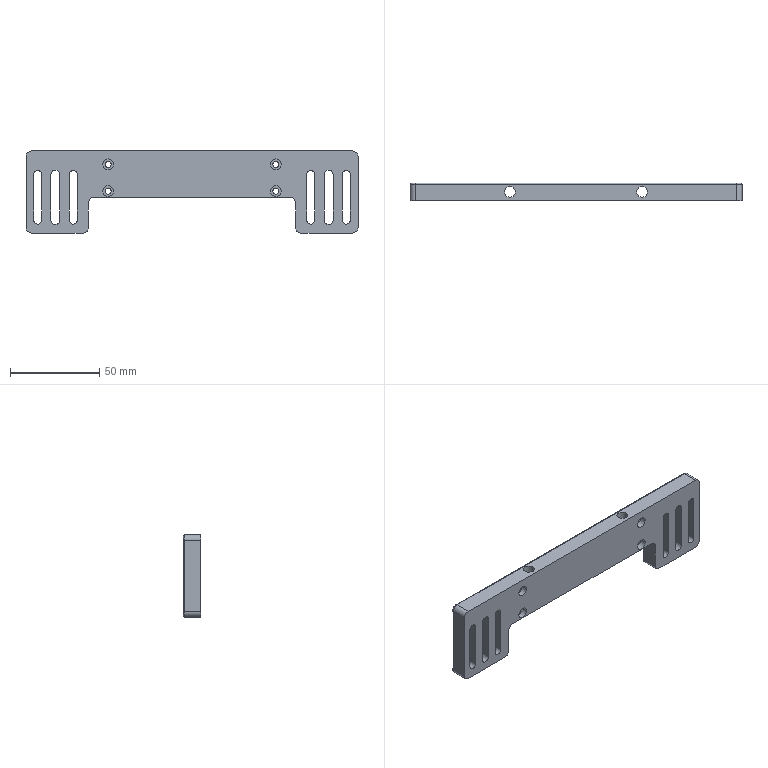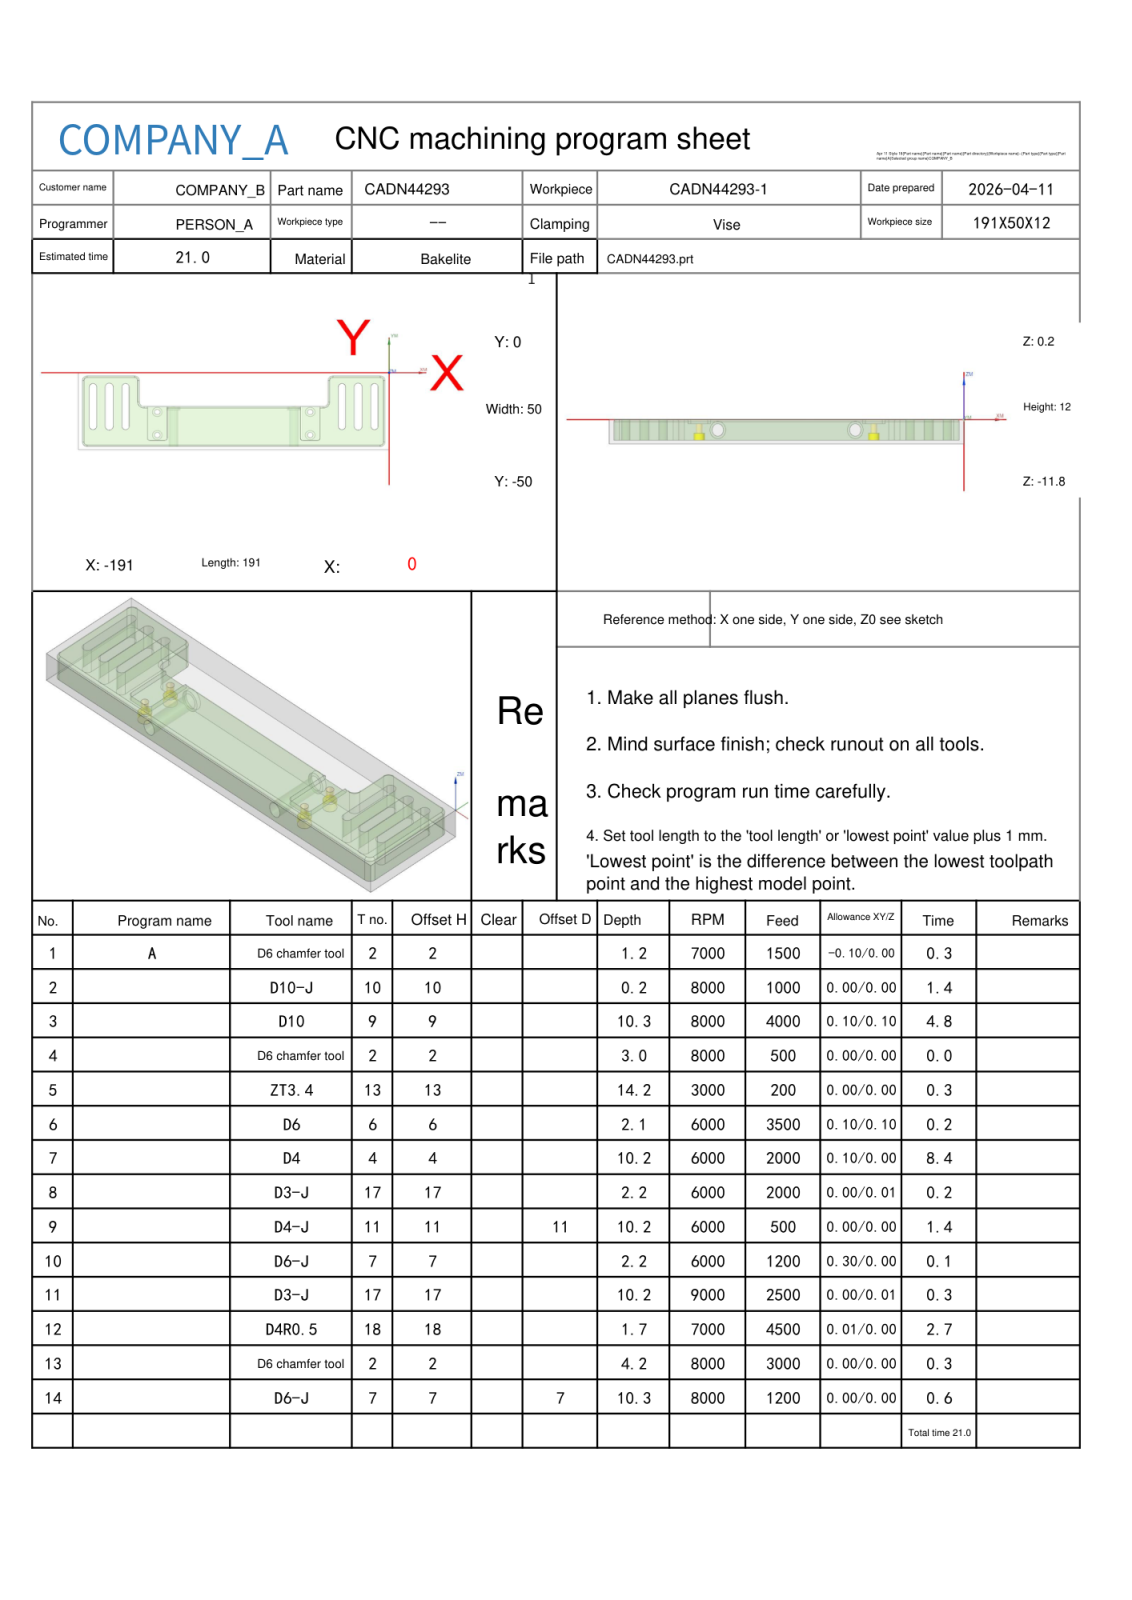NC program | NX | posted by the shop | part box 186 x 10 x 46 mm
Lines 1588 to 2413 of 7485:
N7 T04 M06
(D4  D=4. R=0. H=04 ce=0.10 di=0.00)
G00 G90 G54 X-18.6 Y-22. M03 S6000
G43 H04 Z20.
M08
Z.5
G01 Y-9.25 Z.464 F2000.
G03 X-18.76 Y-8.93 Z.463 I-.4 J0.0
X-19. Y-8.85 Z.463 I-.24 J-.32
X-19.4 Y-9.25 Z.461 I0.0 J-.4
G01 Y-34.75 Z.389
G03 X-19. Y-35.15 Z.388 I.4 J0.0
X-18.6 Y-34.75 Z.386 I0.0 J.4
G01 Y-9.25 Z.314
G03 X-18.76 Y-8.93 Z.313 I-.4 J0.0
X-19. Y-8.85 Z.313 I-.24 J-.32
X-19.4 Y-9.25 Z.311 I0.0 J-.4
G01 Y-34.75 Z.239
G03 X-19. Y-35.15 Z.238 I.4 J0.0
X-18.6 Y-34.75 Z.236 I0.0 J.4
G01 Y-9.25 Z.164
G03 X-18.76 Y-8.93 Z.163 I-.4 J0.0
X-19. Y-8.85 Z.163 I-.24 J-.32
X-19.4 Y-9.25 Z.161 I0.0 J-.4
G01 Y-34.75 Z.089
G03 X-19. Y-35.15 Z.088 I.4 J0.0
X-18.6 Y-34.75 Z.086 I0.0 J.4
G01 Y-9.25 Z.014
G03 X-18.76 Y-8.93 Z.013 I-.4 J0.0
X-19. Y-8.85 Z.013 I-.24 J-.32
X-19.4 Y-9.25 Z.011 I0.0 J-.4
G01 Y-34.75 Z-.061
G03 X-19. Y-35.15 Z-.063 I.4 J0.0
X-18.6 Y-34.75 Z-.064 I0.0 J.4
G01 Y-9.25 Z-.136
G03 X-18.76 Y-8.93 Z-.137 I-.4 J0.0
X-19. Y-8.85 Z-.138 I-.24 J-.32
X-19.4 Y-9.25 Z-.139 I0.0 J-.4
G01 Y-34.75 Z-.211
G03 X-19. Y-35.15 Z-.213 I.4 J0.0
X-18.6 Y-34.75 Z-.214 I0.0 J.4
G01 Y-9.25 Z-.286
G03 X-18.76 Y-8.93 Z-.287 I-.4 J0.0
X-19. Y-8.85 Z-.288 I-.24 J-.32
X-19.4 Y-9.25 Z-.289 I0.0 J-.4
G01 Y-34.75 Z-.361
G03 X-19. Y-35.15 Z-.363 I.4 J0.0
X-18.6 Y-34.75 Z-.364 I0.0 J.4
G01 Y-9.25 Z-.436
G03 X-18.76 Y-8.93 Z-.437 I-.4 J0.0
X-19. Y-8.85 Z-.438 I-.24 J-.32
X-19.4 Y-9.25 Z-.439 I0.0 J-.4
G01 Y-34.75 Z-.511
G03 X-19. Y-35.15 Z-.513 I.4 J0.0
X-18.6 Y-34.75 Z-.514 I0.0 J.4
G01 Y-9.25 Z-.586
G03 X-18.76 Y-8.93 Z-.587 I-.4 J0.0
X-19. Y-8.85 Z-.588 I-.24 J-.32
X-19.4 Y-9.25 Z-.589 I0.0 J-.4
G01 Y-34.75 Z-.661
G03 X-19. Y-35.15 Z-.663 I.4 J0.0
X-18.6 Y-34.75 Z-.664 I0.0 J.4
G01 Y-9.25 Z-.736
G03 X-18.76 Y-8.93 Z-.737 I-.4 J0.0
X-19. Y-8.85 Z-.738 I-.24 J-.32
X-19.4 Y-9.25 Z-.739 I0.0 J-.4
G01 Y-34.75 Z-.811
G03 X-19. Y-35.15 Z-.813 I.4 J0.0
X-18.6 Y-34.75 Z-.814 I0.0 J.4
G01 Y-9.25 Z-.886
G03 X-18.76 Y-8.93 Z-.887 I-.4 J0.0
X-19. Y-8.85 Z-.888 I-.24 J-.32
X-19.4 Y-9.25 Z-.889 I0.0 J-.4
G01 Y-34.75 Z-.961
G03 X-19. Y-35.15 Z-.963 I.4 J0.0
X-18.6 Y-34.75 Z-.964 I0.0 J.4
G01 Y-9.25 Z-1.036
G03 X-18.76 Y-8.93 Z-1.037 I-.4 J0.0
X-19. Y-8.85 Z-1.038 I-.24 J-.32
X-19.4 Y-9.25 Z-1.039 I0.0 J-.4
G01 Y-34.75 Z-1.111
G03 X-19. Y-35.15 Z-1.113 I.4 J0.0
X-18.6 Y-34.75 Z-1.114 I0.0 J.4
G01 Y-9.25 Z-1.186
G03 X-18.76 Y-8.93 Z-1.187 I-.4 J0.0
X-19. Y-8.85 Z-1.188 I-.24 J-.32
X-19.4 Y-9.25 Z-1.189 I0.0 J-.4
G01 Y-34.75 Z-1.261
G03 X-19. Y-35.15 Z-1.263 I.4 J0.0
X-18.6 Y-34.75 Z-1.264 I0.0 J.4
G01 Y-9.25 Z-1.336
G03 X-18.76 Y-8.93 Z-1.337 I-.4 J0.0
X-19. Y-8.85 Z-1.338 I-.24 J-.32
X-19.4 Y-9.25 Z-1.339 I0.0 J-.4
G01 Y-34.75 Z-1.411
G03 X-19. Y-35.15 Z-1.413 I.4 J0.0
X-18.6 Y-34.75 Z-1.414 I0.0 J.4
G01 Y-9.25 Z-1.486
G03 X-18.76 Y-8.93 Z-1.487 I-.4 J0.0
X-19. Y-8.85 Z-1.488 I-.24 J-.32
X-19.4 Y-9.25 Z-1.489 I0.0 J-.4
G01 Y-34.75 Z-1.561
G03 X-19. Y-35.15 Z-1.563 I.4 J0.0
X-18.6 Y-34.75 Z-1.564 I0.0 J.4
G01 Y-9.25 Z-1.636
G03 X-18.76 Y-8.93 Z-1.637 I-.4 J0.0
X-19. Y-8.85 Z-1.638 I-.24 J-.32
X-19.4 Y-9.25 Z-1.639 I0.0 J-.4
G01 Y-34.75 Z-1.711
G03 X-19. Y-35.15 Z-1.713 I.4 J0.0
X-18.6 Y-34.75 Z-1.714 I0.0 J.4
G01 Y-9.25 Z-1.786
G03 X-18.76 Y-8.93 Z-1.787 I-.4 J0.0
X-19. Y-8.85 Z-1.788 I-.24 J-.32
X-19.4 Y-9.25 Z-1.789 I0.0 J-.4
G01 Y-34.75 Z-1.861
G03 X-19. Y-35.15 Z-1.863 I.4 J0.0
X-18.6 Y-34.75 Z-1.864 I0.0 J.4
G01 Y-9.25 Z-1.936
G03 X-18.76 Y-8.93 Z-1.937 I-.4 J0.0
X-19. Y-8.85 Z-1.938 I-.24 J-.32
X-19.4 Y-9.25 Z-1.939 I0.0 J-.4
G01 Y-34.75 Z-2.011
G03 X-19. Y-35.15 Z-2.013 I.4 J0.0
X-18.6 Y-34.75 Z-2.014 I0.0 J.4
G01 Y-9.25 Z-2.086
G03 X-18.76 Y-8.93 Z-2.087 I-.4 J0.0
X-19. Y-8.85 Z-2.088 I-.24 J-.32
X-19.4 Y-9.25 Z-2.089 I0.0 J-.4
G01 Y-34.75 Z-2.161
G03 X-19. Y-35.15 Z-2.163 I.4 J0.0
X-18.6 Y-34.75 Z-2.164 I0.0 J.4
G01 Y-9.25 Z-2.236
G03 X-18.76 Y-8.93 Z-2.237 I-.4 J0.0
X-19. Y-8.85 Z-2.238 I-.24 J-.32
X-19.4 Y-9.25 Z-2.239 I0.0 J-.4
G01 Y-34.75 Z-2.311
G03 X-19. Y-35.15 Z-2.313 I.4 J0.0
X-18.6 Y-34.75 Z-2.314 I0.0 J.4
G01 Y-9.25 Z-2.386
G03 X-18.76 Y-8.93 Z-2.387 I-.4 J0.0
X-19. Y-8.85 Z-2.388 I-.24 J-.32
X-19.4 Y-9.25 Z-2.389 I0.0 J-.4
G01 Y-34.75 Z-2.461
G03 X-19. Y-35.15 Z-2.463 I.4 J0.0
X-18.6 Y-34.75 Z-2.464 I0.0 J.4
G01 Y-9.25 Z-2.536
G03 X-18.76 Y-8.93 Z-2.537 I-.4 J0.0
X-19. Y-8.85 Z-2.538 I-.24 J-.32
X-19.4 Y-9.25 Z-2.539 I0.0 J-.4
G01 Y-34.75 Z-2.611
G03 X-19. Y-35.15 Z-2.613 I.4 J0.0
X-18.6 Y-34.75 Z-2.614 I0.0 J.4
G01 Y-9.25 Z-2.686
G03 X-18.76 Y-8.93 Z-2.687 I-.4 J0.0
X-19. Y-8.85 Z-2.688 I-.24 J-.32
X-19.4 Y-9.25 Z-2.689 I0.0 J-.4
G01 Y-34.75 Z-2.761
G03 X-19. Y-35.15 Z-2.763 I.4 J0.0
X-18.6 Y-34.75 Z-2.764 I0.0 J.4
G01 Y-9.25 Z-2.836
G03 X-18.76 Y-8.93 Z-2.837 I-.4 J0.0
X-19. Y-8.85 Z-2.838 I-.24 J-.32
X-19.4 Y-9.25 Z-2.839 I0.0 J-.4
G01 Y-34.75 Z-2.911
G03 X-19. Y-35.15 Z-2.913 I.4 J0.0
X-18.6 Y-34.75 Z-2.914 I0.0 J.4
G01 Y-9.25 Z-2.986
G03 X-18.76 Y-8.93 Z-2.987 I-.4 J0.0
X-19. Y-8.85 Z-2.988 I-.24 J-.32
X-19.4 Y-9.25 Z-2.989 I0.0 J-.4
G01 Y-34.75 Z-3.061
G03 X-19. Y-35.15 Z-3.063 I.4 J0.0
X-18.6 Y-34.75 Z-3.064 I0.0 J.4
G01 Y-9.25 Z-3.136
G03 X-18.76 Y-8.93 Z-3.137 I-.4 J0.0
X-19. Y-8.85 Z-3.138 I-.24 J-.32
X-19.4 Y-9.25 Z-3.139 I0.0 J-.4
G01 Y-34.75 Z-3.211
G03 X-19. Y-35.15 Z-3.213 I.4 J0.0
X-18.6 Y-34.75 Z-3.214 I0.0 J.4
G01 Y-9.25 Z-3.286
G03 X-18.76 Y-8.93 Z-3.287 I-.4 J0.0
X-19. Y-8.85 Z-3.288 I-.24 J-.32
X-19.4 Y-9.25 Z-3.289 I0.0 J-.4
G01 Y-34.75 Z-3.361
G03 X-19. Y-35.15 Z-3.363 I.4 J0.0
X-18.6 Y-34.75 Z-3.364 I0.0 J.4
G01 Y-9.25 Z-3.436
G03 X-18.76 Y-8.93 Z-3.437 I-.4 J0.0
X-19. Y-8.85 Z-3.438 I-.24 J-.32
X-19.4 Y-9.25 Z-3.439 I0.0 J-.4
G01 Y-34.75 Z-3.511
G03 X-19. Y-35.15 Z-3.513 I.4 J0.0
X-18.6 Y-34.75 Z-3.514 I0.0 J.4
G01 Y-9.25 Z-3.586
G03 X-18.76 Y-8.93 Z-3.587 I-.4 J0.0
X-19. Y-8.85 Z-3.588 I-.24 J-.32
X-19.4 Y-9.25 Z-3.589 I0.0 J-.4
G01 Y-34.75 Z-3.661
G03 X-19. Y-35.15 Z-3.663 I.4 J0.0
X-18.6 Y-34.75 Z-3.664 I0.0 J.4
G01 Y-9.25 Z-3.736
G03 X-18.76 Y-8.93 Z-3.737 I-.4 J0.0
X-19. Y-8.85 Z-3.738 I-.24 J-.32
X-19.4 Y-9.25 Z-3.739 I0.0 J-.4
G01 Y-34.75 Z-3.811
G03 X-19. Y-35.15 Z-3.813 I.4 J0.0
X-18.6 Y-34.75 Z-3.814 I0.0 J.4
G01 Y-9.25 Z-3.886
G03 X-18.76 Y-8.93 Z-3.887 I-.4 J0.0
X-19. Y-8.85 Z-3.888 I-.24 J-.32
X-19.4 Y-9.25 Z-3.889 I0.0 J-.4
G01 Y-34.75 Z-3.961
G03 X-19. Y-35.15 Z-3.963 I.4 J0.0
X-18.6 Y-34.75 Z-3.964 I0.0 J.4
G01 Y-9.25 Z-4.036
G03 X-18.76 Y-8.93 Z-4.037 I-.4 J0.0
X-19. Y-8.85 Z-4.038 I-.24 J-.32
X-19.4 Y-9.25 Z-4.039 I0.0 J-.4
G01 Y-34.75 Z-4.111
G03 X-19. Y-35.15 Z-4.113 I.4 J0.0
X-18.6 Y-34.75 Z-4.114 I0.0 J.4
G01 Y-9.25 Z-4.186
G03 X-18.76 Y-8.93 Z-4.187 I-.4 J0.0
X-19. Y-8.85 Z-4.188 I-.24 J-.32
X-19.4 Y-9.25 Z-4.189 I0.0 J-.4
G01 Y-34.75 Z-4.261
G03 X-19. Y-35.15 Z-4.263 I.4 J0.0
X-18.6 Y-34.75 Z-4.264 I0.0 J.4
G01 Y-9.25 Z-4.336
G03 X-18.76 Y-8.93 Z-4.337 I-.4 J0.0
X-19. Y-8.85 Z-4.338 I-.24 J-.32
X-19.4 Y-9.25 Z-4.339 I0.0 J-.4
G01 Y-34.75 Z-4.411
G03 X-19. Y-35.15 Z-4.413 I.4 J0.0
X-18.6 Y-34.75 Z-4.414 I0.0 J.4
G01 Y-9.25 Z-4.486
G03 X-18.76 Y-8.93 Z-4.487 I-.4 J0.0
X-19. Y-8.85 Z-4.488 I-.24 J-.32
X-19.4 Y-9.25 Z-4.489 I0.0 J-.4
G01 Y-34.75 Z-4.561
G03 X-19. Y-35.15 Z-4.563 I.4 J0.0
X-18.6 Y-34.75 Z-4.564 I0.0 J.4
G01 Y-9.25 Z-4.636
G03 X-18.76 Y-8.93 Z-4.637 I-.4 J0.0
X-19. Y-8.85 Z-4.638 I-.24 J-.32
X-19.4 Y-9.25 Z-4.639 I0.0 J-.4
G01 Y-34.75 Z-4.711
G03 X-19. Y-35.15 Z-4.713 I.4 J0.0
X-18.6 Y-34.75 Z-4.714 I0.0 J.4
G01 Y-9.25 Z-4.786
G03 X-18.76 Y-8.93 Z-4.787 I-.4 J0.0
X-19. Y-8.85 Z-4.788 I-.24 J-.32
X-19.4 Y-9.25 Z-4.789 I0.0 J-.4
G01 Y-34.75 Z-4.861
G03 X-19. Y-35.15 Z-4.863 I.4 J0.0
X-18.6 Y-34.75 Z-4.864 I0.0 J.4
G01 Y-9.25 Z-4.936
G03 X-18.76 Y-8.93 Z-4.937 I-.4 J0.0
X-19. Y-8.85 Z-4.938 I-.24 J-.32
X-19.4 Y-9.25 Z-4.939 I0.0 J-.4
G01 Y-34.75 Z-5.011
G03 X-19. Y-35.15 Z-5.013 I.4 J0.0
X-18.6 Y-34.75 Z-5.014 I0.0 J.4
G01 Y-9.25 Z-5.086
G03 X-18.76 Y-8.93 Z-5.087 I-.4 J0.0
X-19. Y-8.85 Z-5.088 I-.24 J-.32
X-19.4 Y-9.25 Z-5.089 I0.0 J-.4
G01 Y-34.75 Z-5.161
G03 X-19. Y-35.15 Z-5.163 I.4 J0.0
X-18.6 Y-34.75 Z-5.164 I0.0 J.4
G01 Y-9.25 Z-5.236
G03 X-18.76 Y-8.93 Z-5.237 I-.4 J0.0
X-19. Y-8.85 Z-5.238 I-.24 J-.32
X-19.4 Y-9.25 Z-5.239 I0.0 J-.4
G01 Y-34.75 Z-5.311
G03 X-19. Y-35.15 Z-5.313 I.4 J0.0
X-18.6 Y-34.75 Z-5.314 I0.0 J.4
G01 Y-9.25 Z-5.386
G03 X-18.76 Y-8.93 Z-5.387 I-.4 J0.0
X-19. Y-8.85 Z-5.388 I-.24 J-.32
X-19.4 Y-9.25 Z-5.389 I0.0 J-.4
G01 Y-34.75 Z-5.461
G03 X-19. Y-35.15 Z-5.463 I.4 J0.0
X-18.6 Y-34.75 Z-5.464 I0.0 J.4
G01 Y-9.25 Z-5.536
G03 X-18.76 Y-8.93 Z-5.537 I-.4 J0.0
X-19. Y-8.85 Z-5.538 I-.24 J-.32
X-19.4 Y-9.25 Z-5.539 I0.0 J-.4
G01 Y-34.75 Z-5.611
G03 X-19. Y-35.15 Z-5.613 I.4 J0.0
X-18.6 Y-34.75 Z-5.614 I0.0 J.4
G01 Y-9.25 Z-5.686
G03 X-18.76 Y-8.93 Z-5.687 I-.4 J0.0
X-19. Y-8.85 Z-5.688 I-.24 J-.32
X-19.4 Y-9.25 Z-5.689 I0.0 J-.4
G01 Y-34.75 Z-5.761
G03 X-19. Y-35.15 Z-5.763 I.4 J0.0
X-18.6 Y-34.75 Z-5.764 I0.0 J.4
G01 Y-9.25 Z-5.836
G03 X-18.76 Y-8.93 Z-5.837 I-.4 J0.0
X-19. Y-8.85 Z-5.838 I-.24 J-.32
X-19.4 Y-9.25 Z-5.839 I0.0 J-.4
G01 Y-34.75 Z-5.911
G03 X-19. Y-35.15 Z-5.913 I.4 J0.0
X-18.6 Y-34.75 Z-5.914 I0.0 J.4
G01 Y-9.25 Z-5.986
G03 X-18.76 Y-8.93 Z-5.987 I-.4 J0.0
X-19. Y-8.85 Z-5.988 I-.24 J-.32
X-19.4 Y-9.25 Z-5.989 I0.0 J-.4
G01 Y-34.75 Z-6.061
G03 X-19. Y-35.15 Z-6.063 I.4 J0.0
X-18.6 Y-34.75 Z-6.064 I0.0 J.4
G01 Y-9.25 Z-6.136
G03 X-18.76 Y-8.93 Z-6.137 I-.4 J0.0
X-19. Y-8.85 Z-6.138 I-.24 J-.32
X-19.4 Y-9.25 Z-6.139 I0.0 J-.4
G01 Y-34.75 Z-6.211
G03 X-19. Y-35.15 Z-6.213 I.4 J0.0
X-18.6 Y-34.75 Z-6.214 I0.0 J.4
G01 Y-9.25 Z-6.286
G03 X-18.76 Y-8.93 Z-6.287 I-.4 J0.0
X-19. Y-8.85 Z-6.288 I-.24 J-.32
X-19.4 Y-9.25 Z-6.289 I0.0 J-.4
G01 Y-34.75 Z-6.361
G03 X-19. Y-35.15 Z-6.363 I.4 J0.0
X-18.6 Y-34.75 Z-6.364 I0.0 J.4
G01 Y-9.25 Z-6.436
G03 X-18.76 Y-8.93 Z-6.437 I-.4 J0.0
X-19. Y-8.85 Z-6.438 I-.24 J-.32
X-19.4 Y-9.25 Z-6.439 I0.0 J-.4
G01 Y-34.75 Z-6.511
G03 X-19. Y-35.15 Z-6.513 I.4 J0.0
X-18.6 Y-34.75 Z-6.514 I0.0 J.4
G01 Y-9.25 Z-6.586
G03 X-18.76 Y-8.93 Z-6.587 I-.4 J0.0
X-19. Y-8.85 Z-6.588 I-.24 J-.32
X-19.4 Y-9.25 Z-6.589 I0.0 J-.4
G01 Y-34.75 Z-6.661
G03 X-19. Y-35.15 Z-6.663 I.4 J0.0
X-18.6 Y-34.75 Z-6.664 I0.0 J.4
G01 Y-9.25 Z-6.736
G03 X-18.76 Y-8.93 Z-6.737 I-.4 J0.0
X-19. Y-8.85 Z-6.738 I-.24 J-.32
X-19.4 Y-9.25 Z-6.739 I0.0 J-.4
G01 Y-34.75 Z-6.811
G03 X-19. Y-35.15 Z-6.813 I.4 J0.0
X-18.6 Y-34.75 Z-6.814 I0.0 J.4
G01 Y-9.25 Z-6.886
G03 X-18.76 Y-8.93 Z-6.887 I-.4 J0.0
X-19. Y-8.85 Z-6.888 I-.24 J-.32
X-19.4 Y-9.25 Z-6.889 I0.0 J-.4
G01 Y-34.75 Z-6.961
G03 X-19. Y-35.15 Z-6.963 I.4 J0.0
X-18.6 Y-34.75 Z-6.964 I0.0 J.4
G01 Y-9.25 Z-7.036
G03 X-18.76 Y-8.93 Z-7.037 I-.4 J0.0
X-19. Y-8.85 Z-7.038 I-.24 J-.32
X-19.4 Y-9.25 Z-7.039 I0.0 J-.4
G01 Y-34.75 Z-7.111
G03 X-19. Y-35.15 Z-7.113 I.4 J0.0
X-18.6 Y-34.75 Z-7.114 I0.0 J.4
G01 Y-9.25 Z-7.186
G03 X-18.76 Y-8.93 Z-7.187 I-.4 J0.0
X-19. Y-8.85 Z-7.188 I-.24 J-.32
X-19.4 Y-9.25 Z-7.189 I0.0 J-.4
G01 Y-34.75 Z-7.261
G03 X-19. Y-35.15 Z-7.263 I.4 J0.0
X-18.6 Y-34.75 Z-7.264 I0.0 J.4
G01 Y-9.25 Z-7.336
G03 X-18.76 Y-8.93 Z-7.337 I-.4 J0.0
X-19. Y-8.85 Z-7.338 I-.24 J-.32
X-19.4 Y-9.25 Z-7.339 I0.0 J-.4
G01 Y-34.75 Z-7.411
G03 X-19. Y-35.15 Z-7.413 I.4 J0.0
X-18.6 Y-34.75 Z-7.414 I0.0 J.4
G01 Y-9.25 Z-7.486
G03 X-18.76 Y-8.93 Z-7.487 I-.4 J0.0
X-19. Y-8.85 Z-7.488 I-.24 J-.32
X-19.4 Y-9.25 Z-7.489 I0.0 J-.4
G01 Y-34.75 Z-7.561
G03 X-19. Y-35.15 Z-7.563 I.4 J0.0
X-18.6 Y-34.75 Z-7.564 I0.0 J.4
G01 Y-9.25 Z-7.636
G03 X-18.76 Y-8.93 Z-7.637 I-.4 J0.0
X-19. Y-8.85 Z-7.638 I-.24 J-.32
X-19.4 Y-9.25 Z-7.639 I0.0 J-.4
G01 Y-34.75 Z-7.711
G03 X-19. Y-35.15 Z-7.713 I.4 J0.0
X-18.6 Y-34.75 Z-7.714 I0.0 J.4
G01 Y-9.25 Z-7.786
G03 X-18.76 Y-8.93 Z-7.787 I-.4 J0.0
X-19. Y-8.85 Z-7.788 I-.24 J-.32
X-19.4 Y-9.25 Z-7.789 I0.0 J-.4
G01 Y-34.75 Z-7.861
G03 X-19. Y-35.15 Z-7.863 I.4 J0.0
X-18.6 Y-34.75 Z-7.864 I0.0 J.4
G01 Y-9.25 Z-7.936
G03 X-18.76 Y-8.93 Z-7.937 I-.4 J0.0
X-19. Y-8.85 Z-7.938 I-.24 J-.32
X-19.4 Y-9.25 Z-7.939 I0.0 J-.4
G01 Y-34.75 Z-8.011
G03 X-19. Y-35.15 Z-8.013 I.4 J0.0
X-18.6 Y-34.75 Z-8.014 I0.0 J.4
G01 Y-9.25 Z-8.086
G03 X-18.76 Y-8.93 Z-8.087 I-.4 J0.0
X-19. Y-8.85 Z-8.088 I-.24 J-.32
X-19.4 Y-9.25 Z-8.089 I0.0 J-.4
G01 Y-34.75 Z-8.161
G03 X-19. Y-35.15 Z-8.163 I.4 J0.0
X-18.6 Y-34.75 Z-8.164 I0.0 J.4
G01 Y-9.25 Z-8.236
G03 X-18.76 Y-8.93 Z-8.237 I-.4 J0.0
X-19. Y-8.85 Z-8.238 I-.24 J-.32
X-19.4 Y-9.25 Z-8.239 I0.0 J-.4
G01 Y-34.75 Z-8.311
G03 X-19. Y-35.15 Z-8.313 I.4 J0.0
X-18.6 Y-34.75 Z-8.314 I0.0 J.4
G01 Y-9.25 Z-8.386
G03 X-18.76 Y-8.93 Z-8.387 I-.4 J0.0
X-19. Y-8.85 Z-8.388 I-.24 J-.32
X-19.4 Y-9.25 Z-8.389 I0.0 J-.4
G01 Y-34.75 Z-8.461
G03 X-19. Y-35.15 Z-8.463 I.4 J0.0
X-18.6 Y-34.75 Z-8.464 I0.0 J.4
G01 Y-9.25 Z-8.536
G03 X-18.76 Y-8.93 Z-8.537 I-.4 J0.0
X-19. Y-8.85 Z-8.538 I-.24 J-.32
X-19.4 Y-9.25 Z-8.539 I0.0 J-.4
G01 Y-34.75 Z-8.611
G03 X-19. Y-35.15 Z-8.613 I.4 J0.0
X-18.6 Y-34.75 Z-8.614 I0.0 J.4
G01 Y-9.25 Z-8.686
G03 X-18.76 Y-8.93 Z-8.687 I-.4 J0.0
X-19. Y-8.85 Z-8.688 I-.24 J-.32
X-19.4 Y-9.25 Z-8.689 I0.0 J-.4
G01 Y-34.75 Z-8.761
G03 X-19. Y-35.15 Z-8.763 I.4 J0.0
X-18.6 Y-34.75 Z-8.764 I0.0 J.4
G01 Y-9.25 Z-8.836
G03 X-18.76 Y-8.93 Z-8.837 I-.4 J0.0
X-19. Y-8.85 Z-8.838 I-.24 J-.32
X-19.4 Y-9.25 Z-8.839 I0.0 J-.4
G01 Y-34.75 Z-8.911
G03 X-19. Y-35.15 Z-8.913 I.4 J0.0
X-18.6 Y-34.75 Z-8.914 I0.0 J.4
G01 Y-9.25 Z-8.986
G03 X-18.76 Y-8.93 Z-8.987 I-.4 J0.0
X-19. Y-8.85 Z-8.988 I-.24 J-.32
X-19.4 Y-9.25 Z-8.989 I0.0 J-.4
G01 Y-34.75 Z-9.061
G03 X-19. Y-35.15 Z-9.063 I.4 J0.0
X-18.6 Y-34.75 Z-9.064 I0.0 J.4
G01 Y-9.25 Z-9.136
G03 X-18.76 Y-8.93 Z-9.137 I-.4 J0.0
X-19. Y-8.85 Z-9.138 I-.24 J-.32
X-19.4 Y-9.25 Z-9.139 I0.0 J-.4
G01 Y-34.75 Z-9.211
G03 X-19. Y-35.15 Z-9.213 I.4 J0.0
X-18.6 Y-34.75 Z-9.214 I0.0 J.4
G01 Y-9.25 Z-9.286
G03 X-18.76 Y-8.93 Z-9.287 I-.4 J0.0
X-19. Y-8.85 Z-9.288 I-.24 J-.32
X-19.4 Y-9.25 Z-9.289 I0.0 J-.4
G01 Y-34.75 Z-9.361
G03 X-19. Y-35.15 Z-9.363 I.4 J0.0
X-18.6 Y-34.75 Z-9.364 I0.0 J.4
G01 Y-9.25 Z-9.436
G03 X-18.76 Y-8.93 Z-9.437 I-.4 J0.0
X-19. Y-8.85 Z-9.438 I-.24 J-.32
X-19.4 Y-9.25 Z-9.439 I0.0 J-.4
G01 Y-34.75 Z-9.511
G03 X-19. Y-35.15 Z-9.513 I.4 J0.0
X-18.6 Y-34.75 Z-9.514 I0.0 J.4
G01 Y-9.25 Z-9.586
G03 X-18.76 Y-8.93 Z-9.587 I-.4 J0.0
X-19. Y-8.85 Z-9.588 I-.24 J-.32
X-19.4 Y-9.25 Z-9.589 I0.0 J-.4
G01 Y-34.75 Z-9.661
G03 X-19. Y-35.15 Z-9.663 I.4 J0.0
X-18.6 Y-34.75 Z-9.664 I0.0 J.4
G01 Y-9.25 Z-9.736
G03 X-18.76 Y-8.93 Z-9.737 I-.4 J0.0
X-19. Y-8.85 Z-9.738 I-.24 J-.32
X-19.4 Y-9.25 Z-9.739 I0.0 J-.4
G01 Y-34.75 Z-9.811
G03 X-19. Y-35.15 Z-9.813 I.4 J0.0
X-18.6 Y-34.75 Z-9.814 I0.0 J.4
G01 Y-9.25 Z-9.886
G03 X-18.76 Y-8.93 Z-9.887 I-.4 J0.0
X-19. Y-8.85 Z-9.888 I-.24 J-.32
X-19.4 Y-9.25 Z-9.889 I0.0 J-.4
G01 Y-34.75 Z-9.961
G03 X-19. Y-35.15 Z-9.963 I.4 J0.0
X-18.6 Y-34.75 Z-9.964 I0.0 J.4
G01 Y-22. Z-10.
Y-9.25
G03 X-19. Y-8.85 I-.4 J0.0
X-19.4 Y-9.25 I0.0 J-.4
G01 Y-34.75
G03 X-19. Y-35.15 I.4 J0.0
X-18.6 Y-34.75 I0.0 J.4
G01 Y-22.
Y-21.5
Z-9.
G00 Z20.
X-171.6 Y-22.
Z.5
G01 Y-9.25 Z.465
G03 X-172. Y-8.85 Z.463 I-.4 J0.0
X-172.4 Y-9.25 Z.461 I0.0 J-.4
G01 Y-34.75 Z.391
G03 X-172. Y-35.15 Z.389 I.4 J0.0
X-171.6 Y-34.75 Z.387 I0.0 J.4
G01 Y-9.25 Z.317
G03 X-172. Y-8.85 Z.315 I-.4 J0.0
X-172.4 Y-9.25 Z.313 I0.0 J-.4
G01 Y-34.75 Z.243
G03 X-172. Y-35.15 Z.241 I.4 J0.0
X-171.6 Y-34.75 Z.239 I0.0 J.4
G01 Y-9.25 Z.169
G03 X-172. Y-8.85 Z.167 I-.4 J0.0
X-172.4 Y-9.25 Z.166 I0.0 J-.4
G01 Y-34.75 Z.095
G03 X-172. Y-35.15 Z.093 I.4 J0.0
X-171.6 Y-34.75 Z.092 I0.0 J.4
G01 Y-9.25 Z.021
G03 X-172. Y-8.85 Z.019 I-.4 J0.0
X-172.4 Y-9.25 Z.018 I0.0 J-.4
G01 Y-34.75 Z-.053
G03 X-172. Y-35.15 Z-.055 I.4 J0.0
X-171.6 Y-34.75 Z-.056 I0.0 J.4
G01 Y-9.25 Z-.127
G03 X-172. Y-8.85 Z-.129 I-.4 J0.0
X-172.4 Y-9.25 Z-.13 I0.0 J-.4
G01 Y-34.75 Z-.201
G03 X-172. Y-35.15 Z-.202 I.4 J0.0
X-171.6 Y-34.75 Z-.204 I0.0 J.4
G01 Y-9.25 Z-.275
G03 X-172. Y-8.85 Z-.276 I-.4 J0.0
X-172.4 Y-9.25 Z-.278 I0.0 J-.4
G01 Y-34.75 Z-.349
G03 X-172. Y-35.15 Z-.35 I.4 J0.0
X-171.6 Y-34.75 Z-.352 I0.0 J.4
G01 Y-9.25 Z-.423
G03 X-172. Y-8.85 Z-.424 I-.4 J0.0
X-172.4 Y-9.25 Z-.426 I0.0 J-.4
G01 Y-34.75 Z-.497
G03 X-172. Y-35.15 Z-.498 I.4 J0.0
X-171.6 Y-34.75 Z-.5 I0.0 J.4
G01 Y-9.25 Z-.57
G03 X-172. Y-8.85 Z-.572 I-.4 J0.0
X-172.4 Y-9.25 Z-.574 I0.0 J-.4
G01 Y-34.75 Z-.644
G03 X-172. Y-35.15 Z-.646 I.4 J0.0
X-171.6 Y-34.75 Z-.648 I0.0 J.4
G01 Y-9.25 Z-.718
G03 X-172. Y-8.85 Z-.72 I-.4 J0.0
X-172.4 Y-9.25 Z-.722 I0.0 J-.4
G01 Y-34.75 Z-.792
G03 X-172. Y-35.15 Z-.794 I.4 J0.0
X-171.6 Y-34.75 Z-.796 I0.0 J.4
G01 Y-9.25 Z-.866
G03 X-172. Y-8.85 Z-.868 I-.4 J0.0
X-172.4 Y-9.25 Z-.87 I0.0 J-.4
G01 Y-34.75 Z-.94
G03 X-172. Y-35.15 Z-.942 I.4 J0.0
X-171.6 Y-34.75 Z-.944 I0.0 J.4
G01 Y-9.25 Z-1.014
G03 X-172. Y-8.85 Z-1.016 I-.4 J0.0
X-172.4 Y-9.25 Z-1.018 I0.0 J-.4
G01 Y-34.75 Z-1.088
G03 X-172. Y-35.15 Z-1.09 I.4 J0.0
X-171.6 Y-34.75 Z-1.092 I0.0 J.4
G01 Y-9.25 Z-1.162
G03 X-172. Y-8.85 Z-1.164 I-.4 J0.0
X-172.4 Y-9.25 Z-1.165 I0.0 J-.4
G01 Y-34.75 Z-1.236
G03 X-172. Y-35.15 Z-1.238 I.4 J0.0
X-171.6 Y-34.75 Z-1.239 I0.0 J.4
G01 Y-9.25 Z-1.31
G03 X-172. Y-8.85 Z-1.312 I-.4 J0.0
X-172.4 Y-9.25 Z-1.313 I0.0 J-.4
G01 Y-34.75 Z-1.384
G03 X-172. Y-35.15 Z-1.386 I.4 J0.0
X-171.6 Y-34.75 Z-1.387 I0.0 J.4
G01 Y-9.25 Z-1.458
G03 X-172. Y-8.85 Z-1.46 I-.4 J0.0
X-172.4 Y-9.25 Z-1.461 I0.0 J-.4
G01 Y-34.75 Z-1.532
G03 X-172. Y-35.15 Z-1.533 I.4 J0.0
X-171.6 Y-34.75 Z-1.535 I0.0 J.4
G01 Y-9.25 Z-1.606
G03 X-172. Y-8.85 Z-1.607 I-.4 J0.0
X-172.4 Y-9.25 Z-1.609 I0.0 J-.4
G01 Y-34.75 Z-1.68
G03 X-172. Y-35.15 Z-1.681 I.4 J0.0
X-171.6 Y-34.75 Z-1.683 I0.0 J.4
G01 Y-9.25 Z-1.754
G03 X-172. Y-8.85 Z-1.755 I-.4 J0.0
X-172.4 Y-9.25 Z-1.757 I0.0 J-.4
G01 Y-34.75 Z-1.827
G03 X-172. Y-35.15 Z-1.829 I.4 J0.0
X-171.6 Y-34.75 Z-1.831 I0.0 J.4
G01 Y-9.25 Z-1.901
G03 X-172. Y-8.85 Z-1.903 I-.4 J0.0
X-172.4 Y-9.25 Z-1.905 I0.0 J-.4
G01 Y-34.75 Z-1.975
G03 X-172. Y-35.15 Z-1.977 I.4 J0.0
X-171.6 Y-34.75 Z-1.979 I0.0 J.4
G01 Y-9.25 Z-2.049
G03 X-172. Y-8.85 Z-2.051 I-.4 J0.0
X-172.4 Y-9.25 Z-2.053 I0.0 J-.4
G01 Y-34.75 Z-2.123
G03 X-172. Y-35.15 Z-2.125 I.4 J0.0
X-171.6 Y-34.75 Z-2.127 I0.0 J.4
G01 Y-9.25 Z-2.197
G03 X-172. Y-8.85 Z-2.199 I-.4 J0.0
X-172.4 Y-9.25 Z-2.201 I0.0 J-.4
G01 Y-34.75 Z-2.271
G03 X-172. Y-35.15 Z-2.273 I.4 J0.0
X-171.6 Y-34.75 Z-2.275 I0.0 J.4
G01 Y-9.25 Z-2.345
G03 X-172. Y-8.85 Z-2.347 I-.4 J0.0
X-172.4 Y-9.25 Z-2.349 I0.0 J-.4
G01 Y-34.75 Z-2.419
G03 X-172. Y-35.15 Z-2.421 I.4 J0.0
X-171.6 Y-34.75 Z-2.423 I0.0 J.4
G01 Y-9.25 Z-2.493
G03 X-172. Y-8.85 Z-2.495 I-.4 J0.0
X-172.4 Y-9.25 Z-2.496 I0.0 J-.4
G01 Y-34.75 Z-2.567
G03 X-172. Y-35.15 Z-2.569 I.4 J0.0
X-171.6 Y-34.75 Z-2.57 I0.0 J.4
G01 Y-9.25 Z-2.641
G03 X-172. Y-8.85 Z-2.643 I-.4 J0.0
X-172.4 Y-9.25 Z-2.644 I0.0 J-.4
G01 Y-34.75 Z-2.715
G03 X-172. Y-35.15 Z-2.717 I.4 J0.0
X-171.6 Y-34.75 Z-2.718 I0.0 J.4
G01 Y-9.25 Z-2.789
G03 X-172. Y-8.85 Z-2.79 I-.4 J0.0
X-172.4 Y-9.25 Z-2.792 I0.0 J-.4
G01 Y-34.75 Z-2.863
G03 X-172. Y-35.15 Z-2.864 I.4 J0.0
X-171.6 Y-34.75 Z-2.866 I0.0 J.4
G01 Y-9.25 Z-2.937
G03 X-172. Y-8.85 Z-2.938 I-.4 J0.0
X-172.4 Y-9.25 Z-2.94 I0.0 J-.4
G01 Y-34.75 Z-3.011
G03 X-172. Y-35.15 Z-3.012 I.4 J0.0
X-171.6 Y-34.75 Z-3.014 I0.0 J.4
G01 Y-9.25 Z-3.085
G03 X-172. Y-8.85 Z-3.086 I-.4 J0.0
X-172.4 Y-9.25 Z-3.088 I0.0 J-.4
G01 Y-34.75 Z-3.158
G03 X-172. Y-35.15 Z-3.16 I.4 J0.0
X-171.6 Y-34.75 Z-3.162 I0.0 J.4
G01 Y-9.25 Z-3.232
G03 X-172. Y-8.85 Z-3.234 I-.4 J0.0
X-172.4 Y-9.25 Z-3.236 I0.0 J-.4
G01 Y-34.75 Z-3.306
G03 X-172. Y-35.15 Z-3.308 I.4 J0.0
X-171.6 Y-34.75 Z-3.31 I0.0 J.4
G01 Y-9.25 Z-3.38
G03 X-172. Y-8.85 Z-3.382 I-.4 J0.0
X-172.4 Y-9.25 Z-3.384 I0.0 J-.4
G01 Y-34.75 Z-3.454
G03 X-172. Y-35.15 Z-3.456 I.4 J0.0
X-171.6 Y-34.75 Z-3.458 I0.0 J.4
G01 Y-9.25 Z-3.528
G03 X-172. Y-8.85 Z-3.53 I-.4 J0.0
X-172.4 Y-9.25 Z-3.532 I0.0 J-.4
G01 Y-34.75 Z-3.602
G03 X-172. Y-35.15 Z-3.604 I.4 J0.0
X-171.6 Y-34.75 Z-3.606 I0.0 J.4
G01 Y-9.25 Z-3.676
G03 X-172. Y-8.85 Z-3.678 I-.4 J0.0
X-172.4 Y-9.25 Z-3.68 I0.0 J-.4
G01 Y-34.75 Z-3.75
G03 X-172. Y-35.15 Z-3.752 I.4 J0.0
X-171.6 Y-34.75 Z-3.753 I0.0 J.4
G01 Y-9.25 Z-3.824
G03 X-172. Y-8.85 Z-3.826 I-.4 J0.0
X-172.4 Y-9.25 Z-3.827 I0.0 J-.4
G01 Y-34.75 Z-3.898
G03 X-172. Y-35.15 Z-3.9 I.4 J0.0
X-171.6 Y-34.75 Z-3.901 I0.0 J.4
G01 Y-9.25 Z-3.972
G03 X-172. Y-8.85 Z-3.974 I-.4 J0.0
X-172.4 Y-9.25 Z-3.975 I0.0 J-.4
G01 Y-34.75 Z-4.046
G03 X-172. Y-35.15 Z-4.048 I.4 J0.0
X-171.6 Y-34.75 Z-4.049 I0.0 J.4
G01 Y-9.25 Z-4.12
G03 X-172. Y-8.85 Z-4.121 I-.4 J0.0
X-172.4 Y-9.25 Z-4.123 I0.0 J-.4
G01 Y-34.75 Z-4.194
G03 X-172. Y-35.15 Z-4.195 I.4 J0.0
X-171.6 Y-34.75 Z-4.197 I0.0 J.4
G01 Y-9.25 Z-4.268
G03 X-172. Y-8.85 Z-4.269 I-.4 J0.0
X-172.4 Y-9.25 Z-4.271 I0.0 J-.4
G01 Y-34.75 Z-4.342
G03 X-172. Y-35.15 Z-4.343 I.4 J0.0
X-171.6 Y-34.75 Z-4.345 I0.0 J.4
G01 Y-9.25 Z-4.416
G03 X-172. Y-8.85 Z-4.417 I-.4 J0.0
X-172.4 Y-9.25 Z-4.419 I0.0 J-.4
G01 Y-34.75 Z-4.489
G03 X-172. Y-35.15 Z-4.491 I.4 J0.0
X-171.6 Y-34.75 Z-4.493 I0.0 J.4
G01 Y-9.25 Z-4.563
G03 X-172. Y-8.85 Z-4.565 I-.4 J0.0
X-172.4 Y-9.25 Z-4.567 I0.0 J-.4
G01 Y-34.75 Z-4.637
G03 X-172. Y-35.15 Z-4.639 I.4 J0.0
X-171.6 Y-34.75 Z-4.641 I0.0 J.4
G01 Y-9.25 Z-4.711
G03 X-172. Y-8.85 Z-4.713 I-.4 J0.0
X-172.4 Y-9.25 Z-4.715 I0.0 J-.4
G01 Y-34.75 Z-4.785
G03 X-172. Y-35.15 Z-4.787 I.4 J0.0
X-171.6 Y-34.75 Z-4.789 I0.0 J.4
G01 Y-9.25 Z-4.859
G03 X-172. Y-8.85 Z-4.861 I-.4 J0.0
X-172.4 Y-9.25 Z-4.863 I0.0 J-.4
G01 Y-34.75 Z-4.933
G03 X-172. Y-35.15 Z-4.935 I.4 J0.0
X-171.6 Y-34.75 Z-4.937 I0.0 J.4
G01 Y-9.25 Z-5.007
G03 X-172. Y-8.85 Z-5.009 I-.4 J0.0
X-172.4 Y-9.25 Z-5.011 I0.0 J-.4
G01 Y-34.75 Z-5.081
G03 X-172. Y-35.15 Z-5.083 I.4 J0.0
X-171.6 Y-34.75 Z-5.084 I0.0 J.4
G01 Y-9.25 Z-5.155
G03 X-172. Y-8.85 Z-5.157 I-.4 J0.0
X-172.4 Y-9.25 Z-5.158 I0.0 J-.4
G01 Y-34.75 Z-5.229
G03 X-172. Y-35.15 Z-5.231 I.4 J0.0
X-171.6 Y-34.75 Z-5.232 I0.0 J.4
G01 Y-9.25 Z-5.303
G03 X-172. Y-8.85 Z-5.305 I-.4 J0.0
X-172.4 Y-9.25 Z-5.306 I0.0 J-.4
G01 Y-34.75 Z-5.377
G03 X-172. Y-35.15 Z-5.379 I.4 J0.0
X-171.6 Y-34.75 Z-5.38 I0.0 J.4
G01 Y-9.25 Z-5.451
G03 X-172. Y-8.85 Z-5.452 I-.4 J0.0
X-172.4 Y-9.25 Z-5.454 I0.0 J-.4
G01 Y-34.75 Z-5.525
G03 X-172. Y-35.15 Z-5.526 I.4 J0.0
X-171.6 Y-34.75 Z-5.528 I0.0 J.4
G01 Y-9.25 Z-5.599
G03 X-172. Y-8.85 Z-5.6 I-.4 J0.0
X-172.4 Y-9.25 Z-5.602 I0.0 J-.4
G01 Y-34.75 Z-5.673
G03 X-172. Y-35.15 Z-5.674 I.4 J0.0
X-171.6 Y-34.75 Z-5.676 I0.0 J.4
G01 Y-9.25 Z-5.747
G03 X-172. Y-8.85 Z-5.748 I-.4 J0.0
X-172.4 Y-9.25 Z-5.75 I0.0 J-.4
G01 Y-34.75 Z-5.82
G03 X-172. Y-35.15 Z-5.822 I.4 J0.0
X-171.6 Y-34.75 Z-5.824 I0.0 J.4
G01 Y-9.25 Z-5.894
G03 X-172. Y-8.85 Z-5.896 I-.4 J0.0
X-172.4 Y-9.25 Z-5.898 I0.0 J-.4
G01 Y-34.75 Z-5.968
G03 X-172. Y-35.15 Z-5.97 I.4 J0.0
X-171.6 Y-34.75 Z-5.972 I0.0 J.4
G01 Y-9.25 Z-6.042
G03 X-172. Y-8.85 Z-6.044 I-.4 J0.0
X-172.4 Y-9.25 Z-6.046 I0.0 J-.4
G01 Y-34.75 Z-6.116
G03 X-172. Y-35.15 Z-6.118 I.4 J0.0
X-171.6 Y-34.75 Z-6.12 I0.0 J.4
G01 Y-9.25 Z-6.19
G03 X-172. Y-8.85 Z-6.192 I-.4 J0.0
X-172.4 Y-9.25 Z-6.194 I0.0 J-.4
G01 Y-34.75 Z-6.264
G03 X-172. Y-35.15 Z-6.266 I.4 J0.0
X-171.6 Y-34.75 Z-6.268 I0.0 J.4
G01 Y-9.25 Z-6.338
G03 X-172. Y-8.85 Z-6.34 I-.4 J0.0
X-172.4 Y-9.25 Z-6.342 I0.0 J-.4
G01 Y-34.75 Z-6.412
G03 X-172. Y-35.15 Z-6.414 I.4 J0.0
X-171.6 Y-34.75 Z-6.415 I0.0 J.4
G01 Y-9.25 Z-6.486
G03 X-172. Y-8.85 Z-6.488 I-.4 J0.0
X-172.4 Y-9.25 Z-6.489 I0.0 J-.4
G01 Y-34.75 Z-6.56
G03 X-172. Y-35.15 Z-6.562 I.4 J0.0
X-171.6 Y-34.75 Z-6.563 I0.0 J.4
G01 Y-9.25 Z-6.634
G03 X-172. Y-8.85 Z-6.636 I-.4 J0.0
X-172.4 Y-9.25 Z-6.637 I0.0 J-.4
G01 Y-34.75 Z-6.708
G03 X-172. Y-35.15 Z-6.71 I.4 J0.0
X-171.6 Y-34.75 Z-6.711 I0.0 J.4
G01 Y-9.25 Z-6.782
G03 X-172. Y-8.85 Z-6.783 I-.4 J0.0
X-172.4 Y-9.25 Z-6.785 I0.0 J-.4
G01 Y-34.75 Z-6.856
G03 X-172. Y-35.15 Z-6.857 I.4 J0.0
X-171.6 Y-34.75 Z-6.859 I0.0 J.4
G01 Y-9.25 Z-6.93
G03 X-172. Y-8.85 Z-6.931 I-.4 J0.0
X-172.4 Y-9.25 Z-6.933 I0.0 J-.4
G01 Y-34.75 Z-7.004
G03 X-172. Y-35.15 Z-7.005 I.4 J0.0
X-171.6 Y-34.75 Z-7.007 I0.0 J.4
G01 Y-9.25 Z-7.077
G03 X-172. Y-8.85 Z-7.079 I-.4 J0.0
X-172.4 Y-9.25 Z-7.081 I0.0 J-.4
G01 Y-34.75 Z-7.151
G03 X-172. Y-35.15 Z-7.153 I.4 J0.0
X-171.6 Y-34.75 Z-7.155 I0.0 J.4
G01 Y-9.25 Z-7.225
G03 X-172. Y-8.85 Z-7.227 I-.4 J0.0
X-172.4 Y-9.25 Z-7.229 I0.0 J-.4
G01 Y-34.75 Z-7.299
G03 X-172. Y-35.15 Z-7.301 I.4 J0.0